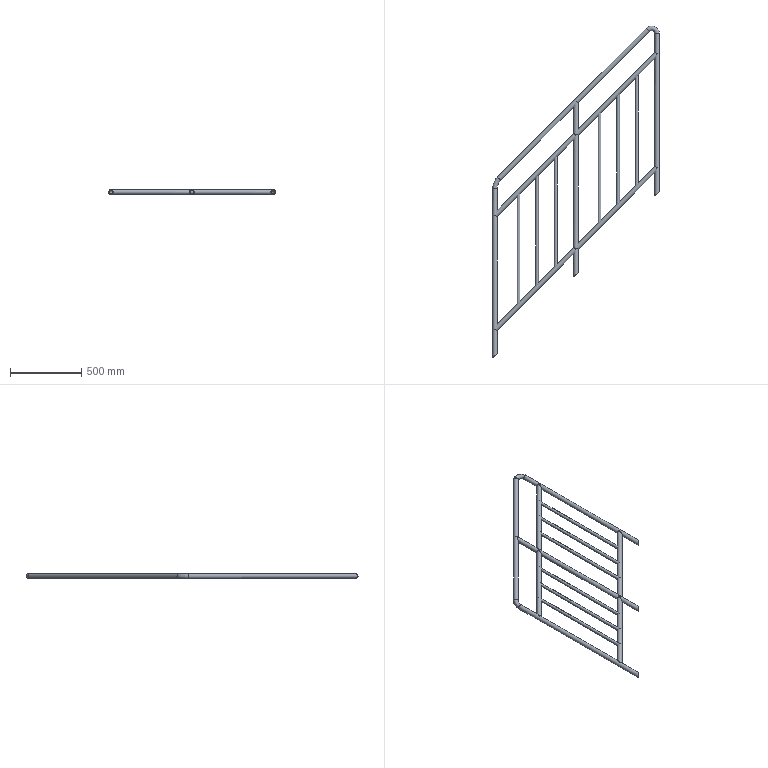Part | STEP file | PN_0015 second-floor stair guardrail A_Default<As Machined> | 16 solids | 64 faces | box 1170 x 2330 x 32 mm | volume 2093979 mm3 | cylinder 37 | plane 23 | torus 4 | commonest cylinder face diameters 32 x17 28 x8 16 x6 20 x6